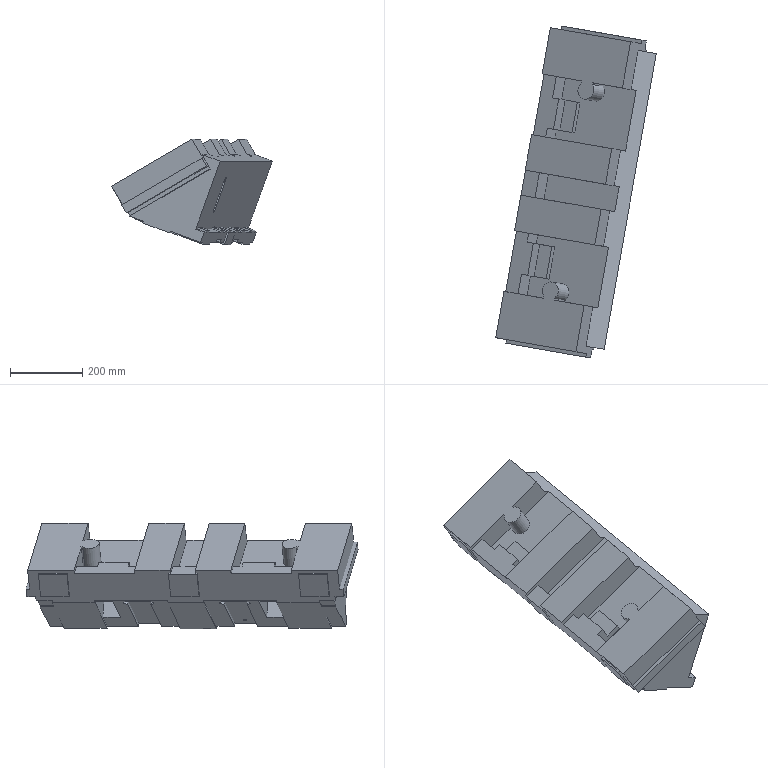Part | NX | features solid 2 | 1 solid | 150 faces | box 443.729 x 917.749 x 291.647 mm | volume 34415700 mm3 | plane 138 | cylinder 11 | cone 1 | commonest cylinder face diameters 20 x4 25 x2 50 x2 60 x2 8.782 x1